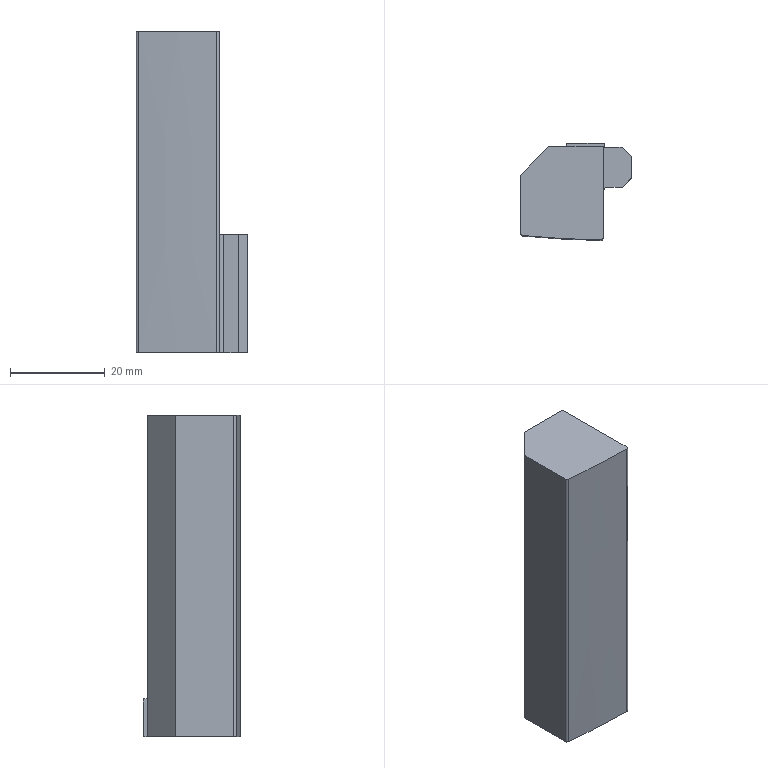Part | STEP file | gslz 2016.10.28-13_id282_x_t | 1 solid | 19 faces | box 23.5 x 20.519 x 68 mm | volume 23024 mm3 | plane 15 | cylinder 3 | other 1 | commonest cylinder face diameters 1 x2 2 x1